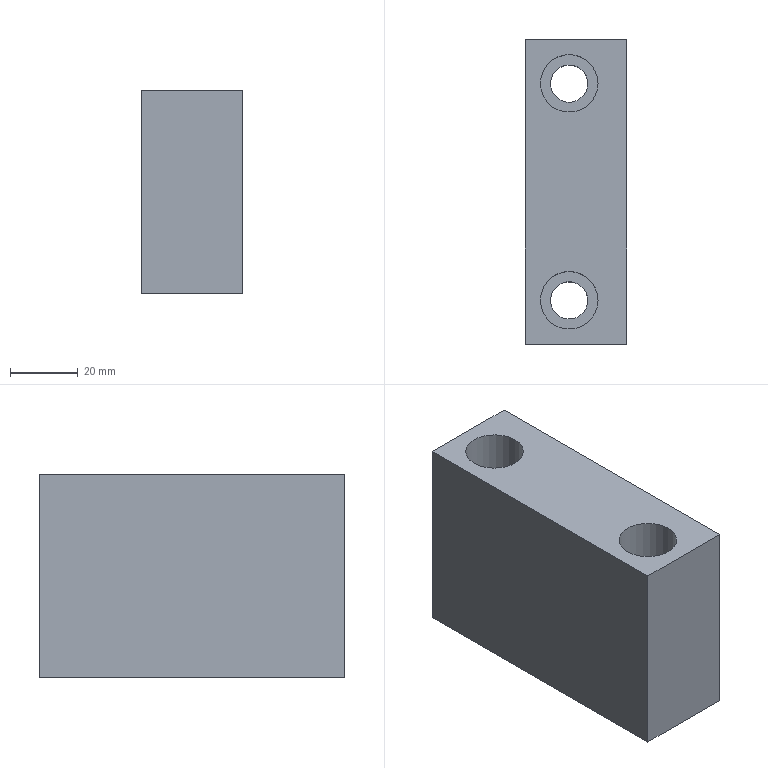Part | STEP file | PN_0004_id1502_x_t | 1 solid | 12 faces | box 30 x 90 x 60 mm | volume 142679 mm3 | plane 8 | cylinder 4 | commonest cylinder face diameters 11 x2 17 x2
STEP:
#1=CARTESIAN_POINT('',(-221.5,-130.,155.));
#2=VERTEX_POINT('',#1);
#3=CARTESIAN_POINT('',(-227.,-130.,155.));
#4=DIRECTION('',(0.,0.,-1.));
#5=DIRECTION('',(1.,0.,0.));
#6=AXIS2_PLACEMENT_3D('',#3,#4,#5);
#7=CIRCLE('',#6,5.5);
#8=EDGE_CURVE('',#2,#2,#7,.T.);
#9=ORIENTED_EDGE('',*,*,#8,.F.);
#10=EDGE_LOOP('',(#9));
#11=FACE_BOUND('',#10,.T.);
#12=CARTESIAN_POINT('',(-221.5,-194.,155.));
#13=VERTEX_POINT('',#12);
#14=CARTESIAN_POINT('',(-227.,-194.,155.));
#15=DIRECTION('',(0.,0.,1.));
#16=DIRECTION('',(1.,0.,0.));
#17=AXIS2_PLACEMENT_3D('',#14,#15,#16);
#18=CIRCLE('',#17,5.5);
#19=EDGE_CURVE('',#13,#13,#18,.T.);
#20=ORIENTED_EDGE('',*,*,#19,.T.);
#21=EDGE_LOOP('',(#20));
#22=FACE_BOUND('',#21,.T.);
#23=CARTESIAN_POINT('',(-210.,-117.,155.));
#24=VERTEX_POINT('',#23);
#25=CARTESIAN_POINT('',(-240.,-117.,155.));
#26=VERTEX_POINT('',#25);
#27=CARTESIAN_POINT('',(-195.,-117.,155.));
#28=DIRECTION('',(-1.,0.,0.));
#29=VECTOR('',#28,1.);
#30=LINE('',#27,#29);
#31=EDGE_CURVE('',#24,#26,#30,.T.);
#32=ORIENTED_EDGE('',*,*,#31,.F.);
#33=CARTESIAN_POINT('',(-210.,-207.,155.));
#34=VERTEX_POINT('',#33);
#35=CARTESIAN_POINT('',(-210.,-7.4,155.));
#36=DIRECTION('',(0.,-1.,0.));
#37=VECTOR('',#36,1.);
#38=LINE('',#35,#37);
#39=EDGE_CURVE('',#24,#34,#38,.T.);
#40=ORIENTED_EDGE('',*,*,#39,.T.);
#41=CARTESIAN_POINT('',(-240.,-207.,155.));
#42=VERTEX_POINT('',#41);
#43=CARTESIAN_POINT('',(-195.,-207.,155.));
#44=DIRECTION('',(1.,0.,0.));
#45=VECTOR('',#44,1.);
#46=LINE('',#43,#45);
#47=EDGE_CURVE('',#42,#34,#46,.T.);
#48=ORIENTED_EDGE('',*,*,#47,.F.);
#49=CARTESIAN_POINT('',(-240.,-229.4,155.));
#50=DIRECTION('',(0.,-1.,0.));
#51=VECTOR('',#50,1.);
#52=LINE('',#49,#51);
#53=EDGE_CURVE('',#26,#42,#52,.T.);
#54=ORIENTED_EDGE('',*,*,#53,.F.);
#55=EDGE_LOOP('',(#32,#40,#48,#54));
#56=FACE_BOUND('',#55,.T.);
#57=CARTESIAN_POINT('',(218.5,-223.,155.));
#58=DIRECTION('',(0.,0.,-1.));
#59=DIRECTION('',(1.,0.,0.));
#60=AXIS2_PLACEMENT_3D('',#57,#58,#59);
#61=PLANE('',#60);
#62=ADVANCED_FACE('',(#11,#22,#56),#61,.T.);
#63=CARTESIAN_POINT('',(-210.,-207.,215.));
#64=VERTEX_POINT('',#63);
#65=CARTESIAN_POINT('',(-210.,-207.,155.));
#66=DIRECTION('',(0.,0.,-1.));
#67=VECTOR('',#66,1.);
#68=LINE('',#65,#67);
#69=EDGE_CURVE('',#64,#34,#68,.T.);
#70=ORIENTED_EDGE('',*,*,#69,.F.);
#71=CARTESIAN_POINT('',(-240.,-207.,215.));
#72=VERTEX_POINT('',#71);
#73=CARTESIAN_POINT('',(-195.,-207.,215.));
#74=DIRECTION('',(-1.,0.,0.));
#75=VECTOR('',#74,1.);
#76=LINE('',#73,#75);
#77=EDGE_CURVE('',#64,#72,#76,.T.);
#78=ORIENTED_EDGE('',*,*,#77,.T.);
#79=CARTESIAN_POINT('',(-240.,-207.,155.));
#80=DIRECTION('',(0.,0.,-1.));
#81=VECTOR('',#80,1.);
#82=LINE('',#79,#81);
#83=EDGE_CURVE('',#72,#42,#82,.T.);
#84=ORIENTED_EDGE('',*,*,#83,.T.);
#85=ORIENTED_EDGE('',*,*,#47,.T.);
#86=EDGE_LOOP('',(#70,#78,#84,#85));
#87=FACE_OUTER_BOUND('',#86,.T.);
#88=CARTESIAN_POINT('',(-195.,-207.,155.));
#89=DIRECTION('',(0.,-1.,0.));
#90=DIRECTION('',(0.,0.,-1.));
#91=AXIS2_PLACEMENT_3D('',#88,#89,#90);
#92=PLANE('',#91);
#93=ADVANCED_FACE('',(#87),#92,.T.);
#94=CARTESIAN_POINT('',(-210.,-117.,215.));
#95=VERTEX_POINT('',#94);
#96=CARTESIAN_POINT('',(-210.,-117.,155.));
#97=DIRECTION('',(0.,0.,1.));
#98=VECTOR('',#97,1.);
#99=LINE('',#96,#98);
#100=EDGE_CURVE('',#24,#95,#99,.T.);
#101=ORIENTED_EDGE('',*,*,#100,.F.);
#102=ORIENTED_EDGE('',*,*,#31,.T.);
#103=CARTESIAN_POINT('',(-240.,-117.,215.));
#104=VERTEX_POINT('',#103);
#105=CARTESIAN_POINT('',(-240.,-117.,138.004));
#106=DIRECTION('',(0.,0.,-1.));
#107=VECTOR('',#106,1.);
#108=LINE('',#105,#107);
#109=EDGE_CURVE('',#104,#26,#108,.T.);
#110=ORIENTED_EDGE('',*,*,#109,.F.);
#111=CARTESIAN_POINT('',(-195.,-117.,215.));
#112=DIRECTION('',(1.,0.,0.));
#113=VECTOR('',#112,1.);
#114=LINE('',#111,#113);
#115=EDGE_CURVE('',#104,#95,#114,.T.);
#116=ORIENTED_EDGE('',*,*,#115,.T.);
#117=EDGE_LOOP('',(#101,#102,#110,#116));
#118=FACE_OUTER_BOUND('',#117,.T.);
#119=CARTESIAN_POINT('',(-195.,-117.,155.));
#120=DIRECTION('',(0.,1.,0.));
#121=DIRECTION('',(0.,0.,1.));
#122=AXIS2_PLACEMENT_3D('',#119,#120,#121);
#123=PLANE('',#122);
#124=ADVANCED_FACE('',(#118),#123,.T.);
#125=CARTESIAN_POINT('',(-235.5,-130.,215.));
#126=VERTEX_POINT('',#125);
#127=CARTESIAN_POINT('',(-227.,-130.,215.));
#128=DIRECTION('',(0.,0.,1.));
#129=DIRECTION('',(-1.,0.,0.));
#130=AXIS2_PLACEMENT_3D('',#127,#128,#129);
#131=CIRCLE('',#130,8.5);
#132=EDGE_CURVE('',#126,#126,#131,.T.);
#133=ORIENTED_EDGE('',*,*,#132,.F.);
#134=EDGE_LOOP('',(#133));
#135=FACE_BOUND('',#134,.T.);
#136=CARTESIAN_POINT('',(-235.5,-194.,215.));
#137=VERTEX_POINT('',#136);
#138=CARTESIAN_POINT('',(-227.,-194.,215.));
#139=DIRECTION('',(0.,0.,-1.));
#140=DIRECTION('',(-1.,0.,0.));
#141=AXIS2_PLACEMENT_3D('',#138,#139,#140);
#142=CIRCLE('',#141,8.5);
#143=EDGE_CURVE('',#137,#137,#142,.T.);
#144=ORIENTED_EDGE('',*,*,#143,.T.);
#145=EDGE_LOOP('',(#144));
#146=FACE_BOUND('',#145,.T.);
#147=CARTESIAN_POINT('',(-210.,-7.4,215.));
#148=DIRECTION('',(0.,-1.,0.));
#149=VECTOR('',#148,1.);
#150=LINE('',#147,#149);
#151=EDGE_CURVE('',#95,#64,#150,.T.);
#152=ORIENTED_EDGE('',*,*,#151,.F.);
#153=ORIENTED_EDGE('',*,*,#115,.F.);
#154=CARTESIAN_POINT('',(-240.,-229.4,215.));
#155=DIRECTION('',(0.,1.,0.));
#156=VECTOR('',#155,1.);
#157=LINE('',#154,#156);
#158=EDGE_CURVE('',#72,#104,#157,.T.);
#159=ORIENTED_EDGE('',*,*,#158,.F.);
#160=ORIENTED_EDGE('',*,*,#77,.F.);
#161=EDGE_LOOP('',(#152,#153,#159,#160));
#162=FACE_BOUND('',#161,.T.);
#163=CARTESIAN_POINT('',(263.5,-223.,215.));
#164=DIRECTION('',(0.,0.,-1.));
#165=DIRECTION('',(1.,0.,0.));
#166=AXIS2_PLACEMENT_3D('',#163,#164,#165);
#167=PLANE('',#166);
#168=ADVANCED_FACE('',(#135,#146,#162),#167,.F.);
#169=ORIENTED_EDGE('',*,*,#158,.T.);
#170=ORIENTED_EDGE('',*,*,#109,.T.);
#171=ORIENTED_EDGE('',*,*,#53,.T.);
#172=ORIENTED_EDGE('',*,*,#83,.F.);
#173=EDGE_LOOP('',(#169,#170,#171,#172));
#174=FACE_OUTER_BOUND('',#173,.T.);
#175=CARTESIAN_POINT('',(-240.,-229.4,138.004));
#176=DIRECTION('',(-1.,0.,0.));
#177=DIRECTION('',(0.,0.,-1.));
#178=AXIS2_PLACEMENT_3D('',#175,#176,#177);
#179=PLANE('',#178);
#180=ADVANCED_FACE('',(#174),#179,.T.);
#181=ORIENTED_EDGE('',*,*,#69,.T.);
#182=ORIENTED_EDGE('',*,*,#39,.F.);
#183=ORIENTED_EDGE('',*,*,#100,.T.);
#184=ORIENTED_EDGE('',*,*,#151,.T.);
#185=EDGE_LOOP('',(#181,#182,#183,#184));
#186=FACE_OUTER_BOUND('',#185,.T.);
#187=CARTESIAN_POINT('',(-210.,-7.4,155.));
#188=DIRECTION('',(1.,0.,0.));
#189=DIRECTION('',(0.,-1.,0.));
#190=AXIS2_PLACEMENT_3D('',#187,#188,#189);
#191=PLANE('',#190);
#192=ADVANCED_FACE('',(#186),#191,.T.);
#193=CARTESIAN_POINT('',(-232.5,-194.,185.));
#194=VERTEX_POINT('',#193);
#195=CARTESIAN_POINT('',(-227.,-194.,185.));
#196=DIRECTION('',(0.,0.,-1.));
#197=DIRECTION('',(-1.,0.,0.));
#198=AXIS2_PLACEMENT_3D('',#195,#196,#197);
#199=CIRCLE('',#198,5.5);
#200=EDGE_CURVE('',#194,#194,#199,.T.);
#201=ORIENTED_EDGE('',*,*,#200,.F.);
#202=EDGE_LOOP('',(#201));
#203=FACE_BOUND('',#202,.T.);
#204=ORIENTED_EDGE('',*,*,#19,.F.);
#205=EDGE_LOOP('',(#204));
#206=FACE_BOUND('',#205,.T.);
#207=CARTESIAN_POINT('',(-227.,-194.,155.));
#208=DIRECTION('',(0.,0.,1.));
#209=DIRECTION('',(1.,0.,0.));
#210=AXIS2_PLACEMENT_3D('',#207,#208,#209);
#211=CYLINDRICAL_SURFACE('',#210,5.5);
#212=ADVANCED_FACE('',(#203,#206),#211,.F.);
#213=ORIENTED_EDGE('',*,*,#200,.T.);
#214=EDGE_LOOP('',(#213));
#215=FACE_BOUND('',#214,.T.);
#216=CARTESIAN_POINT('',(-218.5,-194.,185.));
#217=VERTEX_POINT('',#216);
#218=CARTESIAN_POINT('',(-227.,-194.,185.));
#219=DIRECTION('',(0.,0.,-1.));
#220=DIRECTION('',(1.,0.,0.));
#221=AXIS2_PLACEMENT_3D('',#218,#219,#220);
#222=CIRCLE('',#221,8.5);
#223=EDGE_CURVE('',#217,#217,#222,.T.);
#224=ORIENTED_EDGE('',*,*,#223,.F.);
#225=EDGE_LOOP('',(#224));
#226=FACE_BOUND('',#225,.T.);
#227=CARTESIAN_POINT('',(-227.,-194.,185.));
#228=DIRECTION('',(0.,0.,-1.));
#229=DIRECTION('',(-1.,0.,0.));
#230=AXIS2_PLACEMENT_3D('',#227,#228,#229);
#231=PLANE('',#230);
#232=ADVANCED_FACE('',(#215,#226),#231,.F.);
#233=ORIENTED_EDGE('',*,*,#143,.F.);
#234=EDGE_LOOP('',(#233));
#235=FACE_BOUND('',#234,.T.);
#236=ORIENTED_EDGE('',*,*,#223,.T.);
#237=EDGE_LOOP('',(#236));
#238=FACE_BOUND('',#237,.T.);
#239=CARTESIAN_POINT('',(-227.,-194.,185.));
#240=DIRECTION('',(0.,0.,1.));
#241=DIRECTION('',(1.,0.,0.));
#242=AXIS2_PLACEMENT_3D('',#239,#240,#241);
#243=CYLINDRICAL_SURFACE('',#242,8.5);
#244=ADVANCED_FACE('',(#235,#238),#243,.F.);
#245=CARTESIAN_POINT('',(-232.5,-130.,185.));
#246=VERTEX_POINT('',#245);
#247=CARTESIAN_POINT('',(-227.,-130.,185.));
#248=DIRECTION('',(0.,0.,1.));
#249=DIRECTION('',(-1.,0.,0.));
#250=AXIS2_PLACEMENT_3D('',#247,#248,#249);
#251=CIRCLE('',#250,5.5);
#252=EDGE_CURVE('',#246,#246,#251,.T.);
#253=ORIENTED_EDGE('',*,*,#252,.T.);
#254=EDGE_LOOP('',(#253));
#255=FACE_BOUND('',#254,.T.);
#256=ORIENTED_EDGE('',*,*,#8,.T.);
#257=EDGE_LOOP('',(#256));
#258=FACE_BOUND('',#257,.T.);
#259=CARTESIAN_POINT('',(-227.,-130.,155.));
#260=DIRECTION('',(0.,0.,1.));
#261=DIRECTION('',(1.,0.,0.));
#262=AXIS2_PLACEMENT_3D('',#259,#260,#261);
#263=CYLINDRICAL_SURFACE('',#262,5.5);
#264=ADVANCED_FACE('',(#255,#258),#263,.F.);
#265=ORIENTED_EDGE('',*,*,#252,.F.);
#266=EDGE_LOOP('',(#265));
#267=FACE_BOUND('',#266,.T.);
#268=CARTESIAN_POINT('',(-218.5,-130.,185.));
#269=VERTEX_POINT('',#268);
#270=CARTESIAN_POINT('',(-227.,-130.,185.));
#271=DIRECTION('',(0.,0.,1.));
#272=DIRECTION('',(1.,0.,0.));
#273=AXIS2_PLACEMENT_3D('',#270,#271,#272);
#274=CIRCLE('',#273,8.5);
#275=EDGE_CURVE('',#269,#269,#274,.T.);
#276=ORIENTED_EDGE('',*,*,#275,.T.);
#277=EDGE_LOOP('',(#276));
#278=FACE_BOUND('',#277,.T.);
#279=CARTESIAN_POINT('',(-227.,-130.,185.));
#280=DIRECTION('',(0.,0.,-1.));
#281=DIRECTION('',(-1.,0.,0.));
#282=AXIS2_PLACEMENT_3D('',#279,#280,#281);
#283=PLANE('',#282);
#284=ADVANCED_FACE('',(#267,#278),#283,.F.);
#285=ORIENTED_EDGE('',*,*,#132,.T.);
#286=EDGE_LOOP('',(#285));
#287=FACE_BOUND('',#286,.T.);
#288=ORIENTED_EDGE('',*,*,#275,.F.);
#289=EDGE_LOOP('',(#288));
#290=FACE_BOUND('',#289,.T.);
#291=CARTESIAN_POINT('',(-227.,-130.,185.));
#292=DIRECTION('',(0.,0.,1.));
#293=DIRECTION('',(1.,0.,0.));
#294=AXIS2_PLACEMENT_3D('',#291,#292,#293);
#295=CYLINDRICAL_SURFACE('',#294,8.5);
#296=ADVANCED_FACE('',(#287,#290),#295,.F.);
#297=CLOSED_SHELL('',(#62,#93,#124,#168,#180,#192,#212,#232,#244,#264,#284,#296));
#298=MANIFOLD_SOLID_BREP('',#297);
#299=(LENGTH_UNIT()NAMED_UNIT(*)SI_UNIT(.MILLI.,.METRE.));
#300=UNCERTAINTY_MEASURE_WITH_UNIT(LENGTH_MEASURE(0.00002),#299,'','');
#301=(NAMED_UNIT(*)PLANE_ANGLE_UNIT()SI_UNIT($,.RADIAN.));
#302=PLANE_ANGLE_MEASURE_WITH_UNIT(PLANE_ANGLE_MEASURE(0.01745),#301);
#303=DIMENSIONAL_EXPONENTS(0.,0.,0.,0.,0.,0.,0.);
#304=(CONVERSION_BASED_UNIT('DEGREE',#302)NAMED_UNIT(#303)PLANE_ANGLE_UNIT());
#305=(NAMED_UNIT(*)SI_UNIT($,.STERADIAN.)SOLID_ANGLE_UNIT());
#306=(GEOMETRIC_REPRESENTATION_CONTEXT(3)GLOBAL_UNCERTAINTY_ASSIGNED_CONTEXT((#300))GLOBAL_UNIT_ASSIGNED_CONTEXT((#299,#304,#305))REPRESENTATION_CONTEXT('',''));
#307=ADVANCED_BREP_SHAPE_REPRESENTATION('',(#298),#306);